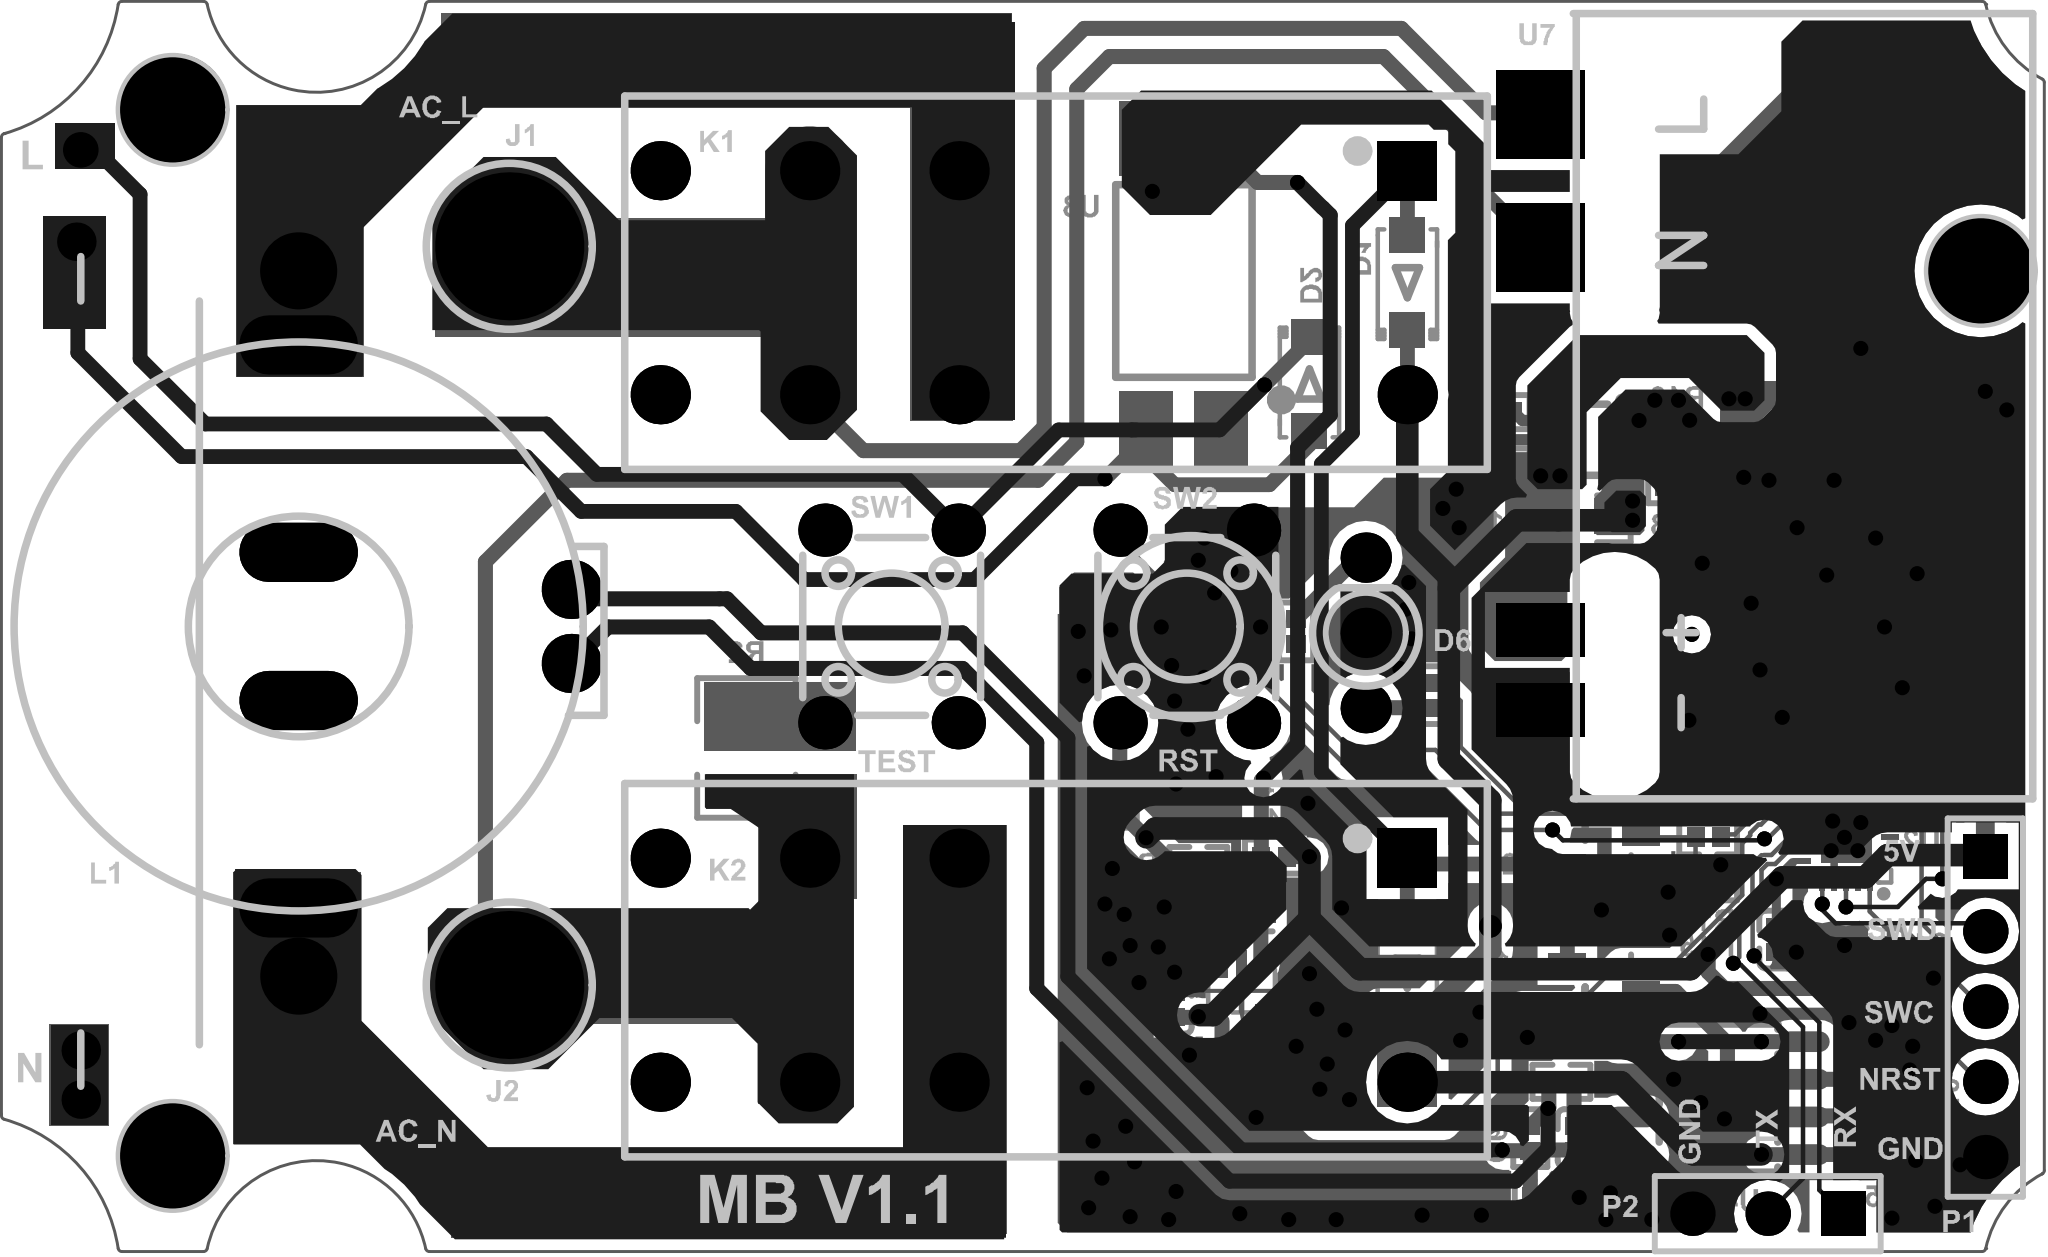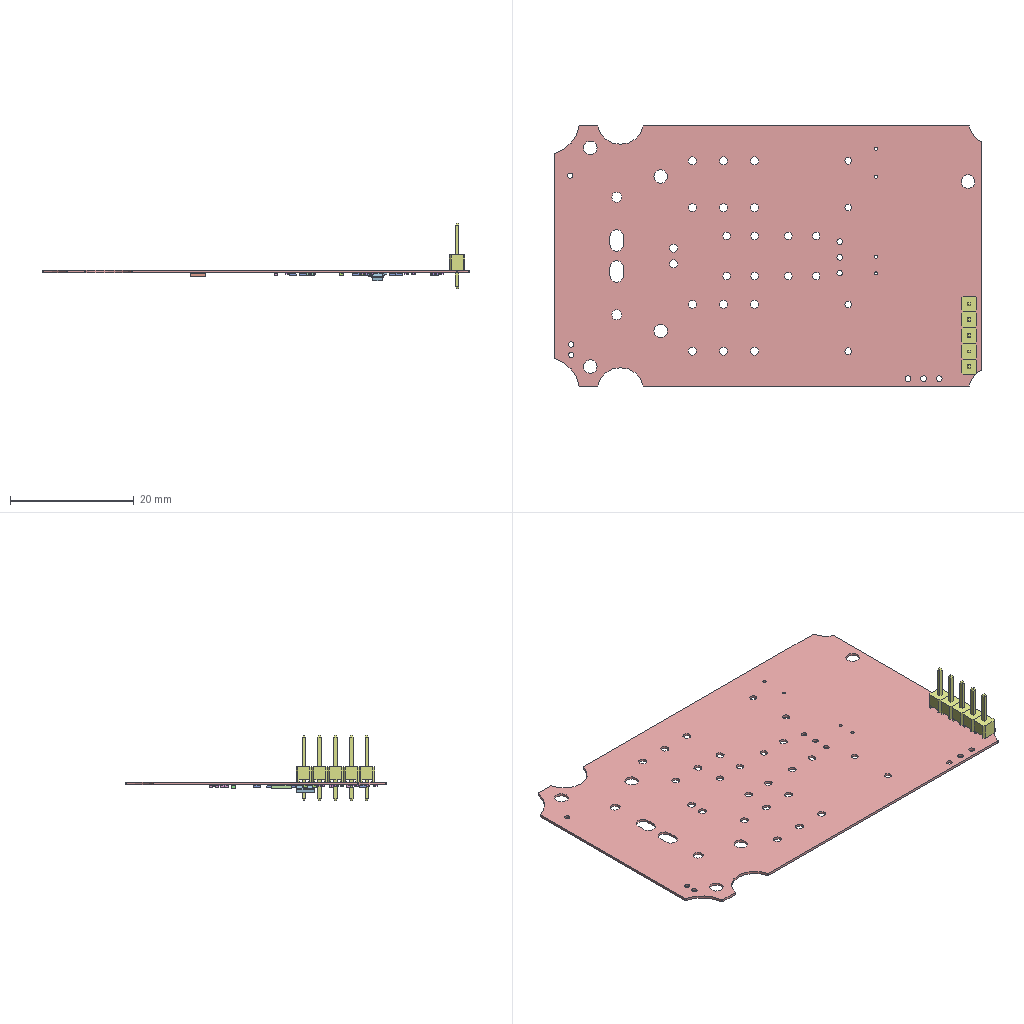Circuit board layout | Altium Designer | box 68.9 x 42.2 x 10.5 mm
Layer stack:
# Altium Designer layer stack of  (unit mm; dielectric type: 0 none, 1 core, 2 prepreg, 3 surface material)
index,name,kind,layer,copper_thickness_mm,dielectric_type,dielectric_thickness_mm,dielectric_material,dielectric_constant
0,Top Paste,other,,,,,,
1,Top Overlay,other,,,,,,
2,Top Solder,dielectric,,,3,0.0102,Solder Resist,3.5
3,Top Layer,copper,Top Layer,0.0356,,,,
4,Dielectric1,dielectric,,,0,0.32,FR-4,4.8
5,Bottom Layer,copper,Bottom Layer,0.0356,,,,
6,Bottom Solder,dielectric,,,3,0.0102,Solder Resist,3.5
7,Bottom Overlay,other,,,,,,
8,Bottom Paste,other,,,,,,
# drill layer pairs: low layer,high layer
drill_pair,Top Layer,Bottom Layer
Part placement:
Designator,Comment,Layer,Footprint,Center-X(mm),Center-Y(mm),Rotation
U7,5V700mA power module, vertical solder,TopLayer,5V700mA电源模块竖直焊接,51.8,28.2,90
P2,Header 3,TopLayer,HDR1X3,59.46,1.15,180
U6,AMS1117-5.0S,BottomLayer,SOT-89-3_L4.5-W2.5-P1.50-LS4.2-BR,62,27.399,180
U5,CJ3439KDW,BottomLayer,SOT-363,53.359,27.268,360
U4,GC54123P-A2,BottomLayer,SOP-8_L5.0-W4.0-P1.27-LS6.2-BL,57.8,5.05,90
U2,PY32F002BF15U6TR,BottomLayer,QFN-20_L3.0-W3.0-P0.40-TL-EP1.7,62.1,13.85,90
U1,MSLMV331IDCKR,BottomLayer,SC-70-5_L2.1-W1.3-P0.65-LS2.3-BL,41.709,8.669,360
R21,10KO (1002) ±1%,BottomLayer,0402_R,37.6,15.15,270
R20,3.3KO (3301) ±1%,BottomLayer,0402_R,48.15,18.65,90
R19,3.3KO (3301) ±1%,BottomLayer,0402_R,43.55,20.8,270
R16,100KO (1003) ±1%,BottomLayer,0402_R,56.4,27.25,180
R15,10KO (1002) ±1%,BottomLayer,0402_R,57.45,12.3,180
R14,1KO (1001) ±1%,BottomLayer,0402_R,51.45,3.7,90
R13,1KO (1001) ±1%,BottomLayer,0402_R,56.4,25.7,180
R12,470O (4700) ±1%,BottomLayer,0402_R,57.45,13.85,180
R11,100O (1000) ±1%,BottomLayer,0402_R,52.5,5.6,360
R10,NC,BottomLayer,0603_R,53.3,24.6,180
R9,100KO (1003) ±1%,BottomLayer,0402_R,50.45,26.4,180
R8,1KO (1001) ±1%,BottomLayer,0402_R,50.45,28.2,180
R6,22KO (2202) ±1%,BottomLayer,0402_R,40.25,11.5,360
R5,22KO (2202) ±1%,BottomLayer,0402_R,40.25,12.95,360
R4,10KO (1002) ±1%,BottomLayer,0402_R,41.9,6,180
R3,22KO (2202) ±1%,BottomLayer,0402_R,42.8,13.2,360
R1,10KO (1002) ±1%,BottomLayer,0402_R,63.15,8.75,180
Q2,9013,BottomLayer,SOT-23(SOT-23-3),53.95,12.95,360
Q1,MCR100-6,BottomLayer,SOT-23-3_L2.9-W1.3-P1.90-LS2.4-BR,53.95,9.6,360
P1,Single-row 2.54 pin header-5P,TopLayer,HDR1X5,66.8,8.14,270
C12,1.0uF (105) 10% 25V,BottomLayer,0402_C,58.65,27.15,90
C11,1.0uF (105) 10% 25V,BottomLayer,0402_C,66.8,27.85,270
C10,47nF (473) 10% 50V,BottomLayer,0402_C,64.25,4.85,270
C9,47nF (473) 10% 50V,BottomLayer,0402_C,51.9,1.7,180
C8,47nF (473) 10% 50V,BottomLayer,0402_C,52.5,7.1,360
C7,47nF (473) 10% 50V,BottomLayer,0402_C,62.8,4.9,270
C6,1.0uF (105) 10% 25V,BottomLayer,0402_C,52.95,3.7,270
C5,100nF (104) 10% 50V,BottomLayer,0402_C,63.35,2.95,180
C4,2.2uF (225) 10% 16V,BottomLayer,0603_C,43.159,11.468,360
C3,100nF (104) 10% 50V,BottomLayer,0402_C,59.75,10.4,270
C2,100nF (104) 10% 50V,BottomLayer,0402_C,39.45,8.2,90
C1,100nF (104) 10% 50V,BottomLayer,0402_C,63.1,10.2,180
D6,Common-cathode bicolour LED,TopLayer,LED_3MM-2P,45.9,20.75,90
U3,PC817CS,BottomLayer,SOP-4_L6.5-W4.6-P2.54-LS10.2-BL,39.75,32.55,180
D2,A7,BottomLayer,SOD-123FL_L2.8-W1.8-LS3.7-RD,44,29.15,270
SW2,Through-hole push button 6X6,TopLayer,SW-TH_4P-L6.0-W6.0-P4.50-LS6.5,39.862,20.967,90
K2,HF115F/012-1ZS3,TopLayer,RELAY-TH_HF115F-012-1ZS3,34.7,9.367,180
R2,15K 1%,BottomLayer,1210_R,25.005,16.867,90
SW1,Through-hole push button 6X6,TopLayer,SW-TH_4P-L6.0-W6.0-P4.50-LS6.5,29.905,20.968,90
L1,ZCT56-06N-01,TopLayer,ZCT56-06N-01,14.5,20.968,90
K1,HF115F/012-1ZS3,TopLayer,RELAY-TH_HF115F-012-1ZS3,34.7,32.568,180
J2,Wire solder point, type E,TopLayer,焊线点E型,17.005,8.867,90
J1,Wire solder point, type E,TopLayer,焊线点E型,17.005,33.796,90
D3,A7,BottomLayer,SOD-123FL_L2.8-W1.8-LS3.7-RD,47.3,9.268,90
D1,A7,BottomLayer,SOD-123FL_L2.8-W1.8-LS3.7-RD,47.305,32.568,90
Pad and via stacks:
# Altium Designer via and pad stacks of  (unit mm). Each distinct definition once, with the count of objects using it.
# via: kind,start_layer,end_layer,hole_mm,diameter_mm,mode(0 simple;1 top-mid-bottom;2 full stack),diameter_per_layer,count,example_net
# pad: kind,layer,hole_mm,hole_type(0 round;1 square;2 slot),plating,top_size,top_shape(1 round;2 rect;3 octagon;9 rounded rect),mid_size,bottom_size,mode,footprint,size_per_layer,count,example
pad,Multi-Layer,0.5,0,plated,1.8x3,2,1.8x3,1.8x3,0,5V700mA\u00B5\u00E7\u00D4\u00B4\u00C4\u00A3\u00BF\u00E9\u00CA\u00FA\u00D6\u00B1\u00BA\u00B8\u00BD\u00D3,,2,U7.2
pad,Multi-Layer,0.5,0,plated,3x3,2,3x3,3x3,0,5V700mA\u00B5\u00E7\u00D4\u00B4\u00C4\u00A3\u00BF\u00E9\u00CA\u00FA\u00D6\u00B1\u00BA\u00B8\u00BD\u00D3,,2,U7.4
pad,Multi-Layer,0.9,0,plated,1.5x1.5,2,1.5x1.5,1.5x1.5,0,HDR1X3,,1,P2.1
pad,Multi-Layer,0.9,0,plated,1.5x1.5,1,1.5x1.5,1.5x1.5,0,HDR1X3,,2,P2.2
pad,Multi-Layer,0.85,0,plated,1.3x1.3,1,1.3x1.3,1.3x1.3,0,,,3,1
pad,Multi-Layer,0.9,0,plated,1.7x1.7,1,1.7x1.7,1.7x1.7,0,LED 3MM-2P,,3,D6.2
pad,Multi-Layer,1.2,0,plated,1.8x1.8,1,1.8x1.8,1.8x1.8,0,SW-TH_4P-L6.0-W6.0-P4.50-LS6.5,,8,SW2.4
pad,Multi-Layer,2.2,0,plated,5x5,1,5x5,5x5,0,\u00BA\u00B8\u00CF\u00DF\u00B5\u00E3E\u00D0\u00CD,,2,J2.1
pad,Multi-Layer,1.1,0,plated,2x2,1,2x2,2x2,0,RELAY-TH_HF115F-012-1ZS3,,2,K2.8
pad,Multi-Layer,1.3,0,plated,2x2,1,2x2,2x2,0,RELAY-TH_HF115F-012-1ZS3,,12,K2.7
pad,Multi-Layer,1.1,0,plated,2x2,2,2x2,2x2,0,RELAY-TH_HF115F-012-1ZS3,,2,K2.1
pad,Multi-Layer,1.3,0,plated,2x2,1,2x2,2x2,0,ZCT56-06N-01,,2,L1.6
pad,Multi-Layer,1.6,0,plated,4x2,1,4x2,4x2,0,ZCT56-06N-01,,2,L1.2
pad,Multi-Layer,2.2,2,plated,4x2,1,4x2,4x2,0,ZCT56-06N-01,,2,L1.3
pad,Multi-Layer,2.2,0,plated,3.7x3.7,1,3.7x3.7,3.7x3.7,0,,,3,0
pad,Multi-Layer,0.9,0,plated,1.5x1.5,1,1.5x1.5,1.5x1.5,0,HDR1X5,,4,P1.3
pad,Multi-Layer,0.9,0,plated,1.5x1.5,2,1.5x1.5,1.5x1.5,0,HDR1X5,,1,P1.1
pad,Bottom Layer,0,0,plated,1.575x0.6731,2,1.575x0.6731,1.575x0.6731,0,SOT-89-3_L4.5-W2.5-P1.50-LS4.2-BR,,2,U6.1
pad,Bottom Layer,0,0,plated,1.141x1.141,1,1.141x1.141,1.141x1.141,0,SOT-89-3_L4.5-W2.5-P1.50-LS4.2-BR,,1,U6.2
pad,Bottom Layer,0,0,plated,1.2x1.2,2,1.2x1.2,1.2x1.2,0,SOD-123FL_L2.8-W1.8-LS3.7-RD,,6,D2.2
pad,Bottom Layer,0,0,plated,1.8x2.5,2,1.8x2.5,1.8x2.5,0,SOP-4_L6.5-W4.6-P2.54-LS10.2-BL,,4,U3.4
pad,Bottom Layer,0,0,plated,1.16x2.72,2,1.16x2.72,1.16x2.72,0,1210_R,,2,R2.1
pad,Bottom Layer,0,0,plated,0.6x0.65,2,0.6x0.65,0.6x0.65,0,0402_C,,22,C5.2
pad,Bottom Layer,0,0,plated,0.7x1.7,1,0.7x1.7,0.7x1.7,0,SOP-8_L5.0-W4.0-P1.27-LS6.2-BL,,8,U4.5
pad,Bottom Layer,0,0,plated,0.6x0.65,2,0.6x0.65,0.6x0.65,0,0402_R,,32,R14.1
pad,Bottom Layer,0,0,plated,1.25x0.7,2,1.25x0.7,1.25x0.7,0,SOT-23-3_L2.9-W1.3-P1.90-LS2.4-BR,,3,Q1.3
pad,Bottom Layer,0,0,plated,0.7x1.25,2,0.7x1.25,0.7x1.25,0,SOT-23(SOT-23-3),,3,Q2.3
pad,Bottom Layer,0,0,plated,1.7x1.7,2,1.7x1.7,1.7x1.7,0,QFN-20_L3.0-W3.0-P0.40-TL-EP1.7,,1,U2.21
pad,Bottom Layer,0,0,plated,0.2x0.6,2,0.2x0.6,0.2x0.6,0,QFN-20_L3.0-W3.0-P0.40-TL-EP1.7,,10,U2.20
pad,Bottom Layer,0,0,plated,0.6x0.2,2,0.6x0.2,0.6x0.2,0,QFN-20_L3.0-W3.0-P0.40-TL-EP1.7,,10,U2.15
pad,Bottom Layer,0,0,plated,0.42x1,2,0.42x1,0.42x1,0,SOT-363,,6,U5.1
pad,Bottom Layer,0,0,plated,0.93x0.98,2,0.93x0.98,0.93x0.98,0,0603_R,,2,R10.2
pad,Bottom Layer,0,0,plated,0.93x0.98,2,0.93x0.98,0.93x0.98,0,0603_C,,2,C4.1
pad,Bottom Layer,0,0,plated,0.3505x0.9169,2,0.3505x0.9169,0.3505x0.9169,0,SC-70-5_L2.1-W1.3-P0.65-LS2.3-BL,,5,U1.5
via,Top Layer,Bottom Layer,0.3048,0.508,0,,139,VCC_12V
via,Top Layer,Bottom Layer,0.85,1.2,0,,1,L
via,Top Layer,Bottom Layer,2.2,2.6,0,,2,NetK1_2
via,Top Layer,Bottom Layer,0.381,0.762,0,,1,VCC_12VC1
Copper pours:
name,layer,net,type(0 solid;1 hatched;2 none)
Bottom Layer-No Net,Top Layer,VCC_12V,0
Bottom Layer-No Net,Top Layer,GND,0
Top Layer-NetK2_2,Top Layer,NetK2_2,0
Top Layer-NetK1_2,Top Layer,NetK1_2,0
Top Layer-AC_N,Top Layer,AC_N,0
Top Layer-AC_L,Top Layer,AC_L,0
Bottom Layer-No Net,Top Layer,VCC_12VC1,0
Bottom Layer-No Net,Bottom Layer,VCC_12V,0
Bottom Layer-No Net,Bottom Layer,GND,0
Bottom Layer-No Net,Bottom Layer,VCC_12VC1,0
Bottom Layer-No Net,Bottom Layer,VCC_12V,0
Design rules, without the lines most boards share:
# Altium Designer design rules of  (exported by Altium Designer, unit mm)
# columns: name | kind | enabled | priority | scope1 | scope2 | descriptor | typed fields (field=value)
SilkToSilkClearance | 55 | enabled | 1 | All | All | Silk to Silk (Clearance=0mil) (All),(All) |
SilkToSolderMaskClearance | 54 | enabled | 1 | IsPad | All | Silk To Solder Mask (Clearance=0mil) (IsPad),(All) |
MinimumSolderMaskSliver | 53 | enabled | 1 | All | All | Minimum Solder Mask Sliver (Gap=0mil) (All),(All) |
HoleToHoleClearance | 52 | enabled | 1 | All | All | Hole To Hole Clearance (Gap=0mil) (All),(All) | gap=0
DiffPairsRouting | 51 | enabled | 1 | All | All | Differential Pairs Uncoupled Length using the Gap Constraints (Min=10mil) (Max=10mil) (Prefered=10mil)  and Width Constraints (Min=15mil) (Max=15mil) (Prefered=15mil) (All) |
HoleSize | 42 | enabled | 1 | All | All | Hole Size Constraint (Min=1mil) (Max=500mil) (All) |
ComponentClearance | 24 | disabled | 1 | All | All | Component Clearance Constraint ( Horizontal Gap = 10mil, Vertical Gap = 10mil ) (Disabled)(All),(All)  | gap=0.254
SolderMaskExpansion | 13 | enabled | 1 | All | All | Solder Mask Expansion (Expansion =4mil) (All) | expansion=0.1016
PasteMaskExpansion | 14 | enabled | 1 | All | All | Paste Mask Expansion (Expansion =0mil) (All) | expansion=0
RoutingVias | 11 | enabled | 1 | All | All | Routing Via (MinHoleWidth=12mil) (MaxHoleWidth=12mil) (PreferredHoleWidth=12mil) (MinWidth=20mil) (MaxWidth=20mil) (PreferedWidth=20mil) (All) | via_min_hole=0.3048 via_max_hole=0.3048 via_preferred_diameter=0.508 via_preferred_hole=0.3048
Width | 2 | enabled | 1 | All | All | Width Constraint (Min=6mil) (Max=300mil) (Preferred=10mil) (All) |
PolygonConnect | 20 | enabled | 1 | All | All | Polygon Connect Rule(Direct Connect )(Conductor Width=10mil) (Relief Angle=90 Angle) (Entries=4) (Air Gap Width=10mil) (All),(All) | connect_style(0=relief,1=direct,2=none)=1 relief_conductor_width=0.254 relief_entries=4
PlaneConnect | 6 | enabled | 1 | All | All | Power Plane Connect Rule(Direct Connect )(Expansion=20mil) (Conductor Width=10mil) (Air Gap=10mil) (Entries=4) (All) | relief_conductor_width=0.254 relief_entries=4 relief_expansion=0.508
Clearance | 0 | enabled | 2 | All | All | Clearance Constraint (Gap=6mil) (All),(All) | gap=0.1524
Clearance_1 | 0 | enabled | 1 | inpolygon | All | Clearance Constraint (Gap=6mil) (inpolygon),(All) | gap=0.1524
Classes set for this board:
# Altium Designer classes of  (member kind: 0 net, 1 component, 2 from-to, 3 pad, 4 layer, 5 differential pair, 6 design channel, 7 polygon, 8 structure, 9 xSignal)
# columns: class name | member kind | superclass | members
Leakage-Protection-MB-V1.2 | 1 | no | K1; L1; SW1; J9; J18; K2; SW2; J3; U3; J2; R1; U3; D1; J3; U7; C1; C2; C3; C4; C5; C6; C7; C8; C9; C10; C11; C12; J1; Q1; Q2; R1; R2; R3; R4; R5; R6; R8; R9; R10; R11; R12; R13; R17; R19; R21; U1; U3; U4; U5; U7; U3; D6; D1; R17; U7; D2; D3; P1; R14; R15; R16; R20; U2; U6; P2;